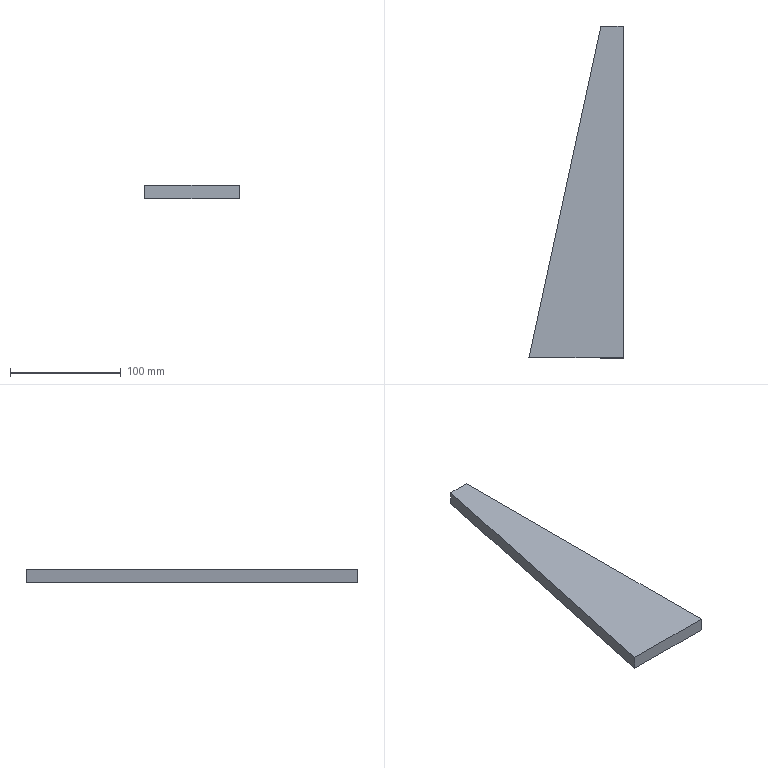Part | SolidWorks | features Extrusion 1 | 1 solid | 6 faces | box 85 x 300 x 12 mm | volume 189000 mm3 | plane 6
STEP:
#1=CARTESIAN_POINT('',(-85.,0.,-6.));
#2=VERTEX_POINT('',#1);
#3=CARTESIAN_POINT('',(0.,0.,-6.));
#4=VERTEX_POINT('',#3);
#5=CARTESIAN_POINT('',(0.,0.,-6.));
#6=DIRECTION('',(1.,0.,0.));
#7=VECTOR('',#6,1000.);
#8=LINE('',#5,#7);
#9=EDGE_CURVE('',#2,#4,#8,.T.);
#10=ORIENTED_EDGE('',*,*,#9,.T.);
#11=CARTESIAN_POINT('',(0.,0.,6.));
#12=VERTEX_POINT('',#11);
#13=CARTESIAN_POINT('',(0.,0.,6.));
#14=DIRECTION('',(0.,0.,-1.));
#15=VECTOR('',#14,1000.);
#16=LINE('',#13,#15);
#17=EDGE_CURVE('',#12,#4,#16,.T.);
#18=ORIENTED_EDGE('',*,*,#17,.F.);
#19=CARTESIAN_POINT('',(-85.,0.,6.));
#20=VERTEX_POINT('',#19);
#21=CARTESIAN_POINT('',(0.,0.,6.));
#22=DIRECTION('',(1.,0.,0.));
#23=VECTOR('',#22,1000.);
#24=LINE('',#21,#23);
#25=EDGE_CURVE('',#20,#12,#24,.T.);
#26=ORIENTED_EDGE('',*,*,#25,.F.);
#27=CARTESIAN_POINT('',(-85.,0.,6.));
#28=DIRECTION('',(0.,0.,-1.));
#29=VECTOR('',#28,1000.);
#30=LINE('',#27,#29);
#31=EDGE_CURVE('',#20,#2,#30,.T.);
#32=ORIENTED_EDGE('',*,*,#31,.T.);
#33=EDGE_LOOP('',(#10,#18,#26,#32));
#34=FACE_OUTER_BOUND('',#33,.T.);
#35=CARTESIAN_POINT('',(0.,0.,6.));
#36=DIRECTION('',(0.,1.,0.));
#37=DIRECTION('',(-1.,0.,0.));
#38=AXIS2_PLACEMENT_3D('',#35,#36,#37);
#39=PLANE('',#38);
#40=ADVANCED_FACE('',(#34),#39,.F.);
#41=CARTESIAN_POINT('',(0.,300.,-6.));
#42=VERTEX_POINT('',#41);
#43=CARTESIAN_POINT('',(0.,0.,-6.));
#44=DIRECTION('',(0.,1.,0.));
#45=VECTOR('',#44,1000.);
#46=LINE('',#43,#45);
#47=EDGE_CURVE('',#4,#42,#46,.T.);
#48=ORIENTED_EDGE('',*,*,#47,.T.);
#49=CARTESIAN_POINT('',(0.,300.,6.));
#50=VERTEX_POINT('',#49);
#51=CARTESIAN_POINT('',(0.,300.,6.));
#52=DIRECTION('',(0.,0.,-1.));
#53=VECTOR('',#52,1000.);
#54=LINE('',#51,#53);
#55=EDGE_CURVE('',#50,#42,#54,.T.);
#56=ORIENTED_EDGE('',*,*,#55,.F.);
#57=CARTESIAN_POINT('',(0.,0.,6.));
#58=DIRECTION('',(0.,1.,0.));
#59=VECTOR('',#58,1000.);
#60=LINE('',#57,#59);
#61=EDGE_CURVE('',#12,#50,#60,.T.);
#62=ORIENTED_EDGE('',*,*,#61,.F.);
#63=ORIENTED_EDGE('',*,*,#17,.T.);
#64=EDGE_LOOP('',(#48,#56,#62,#63));
#65=FACE_OUTER_BOUND('',#64,.T.);
#66=CARTESIAN_POINT('',(0.,0.,6.));
#67=DIRECTION('',(-1.,0.,0.));
#68=DIRECTION('',(0.,0.,1.));
#69=AXIS2_PLACEMENT_3D('',#66,#67,#68);
#70=PLANE('',#69);
#71=ADVANCED_FACE('',(#65),#70,.F.);
#72=CARTESIAN_POINT('',(-20.,300.,-6.));
#73=VERTEX_POINT('',#72);
#74=CARTESIAN_POINT('',(0.,300.,-6.));
#75=DIRECTION('',(-1.,0.,0.));
#76=VECTOR('',#75,1000.);
#77=LINE('',#74,#76);
#78=EDGE_CURVE('',#42,#73,#77,.T.);
#79=ORIENTED_EDGE('',*,*,#78,.T.);
#80=CARTESIAN_POINT('',(-20.,300.,6.));
#81=VERTEX_POINT('',#80);
#82=CARTESIAN_POINT('',(-20.,300.,6.));
#83=DIRECTION('',(0.,0.,-1.));
#84=VECTOR('',#83,1000.);
#85=LINE('',#82,#84);
#86=EDGE_CURVE('',#81,#73,#85,.T.);
#87=ORIENTED_EDGE('',*,*,#86,.F.);
#88=CARTESIAN_POINT('',(0.,300.,6.));
#89=DIRECTION('',(-1.,0.,0.));
#90=VECTOR('',#89,1000.);
#91=LINE('',#88,#90);
#92=EDGE_CURVE('',#50,#81,#91,.T.);
#93=ORIENTED_EDGE('',*,*,#92,.F.);
#94=ORIENTED_EDGE('',*,*,#55,.T.);
#95=EDGE_LOOP('',(#79,#87,#93,#94));
#96=FACE_OUTER_BOUND('',#95,.T.);
#97=CARTESIAN_POINT('',(0.,300.,6.));
#98=DIRECTION('',(0.,-1.,0.));
#99=DIRECTION('',(0.,0.,-1.));
#100=AXIS2_PLACEMENT_3D('',#97,#98,#99);
#101=PLANE('',#100);
#102=ADVANCED_FACE('',(#96),#101,.F.);
#103=CARTESIAN_POINT('',(-20.,300.,-6.));
#104=DIRECTION('',(-0.2118,-0.9773,0.));
#105=VECTOR('',#104,1000.);
#106=LINE('',#103,#105);
#107=EDGE_CURVE('',#73,#2,#106,.T.);
#108=ORIENTED_EDGE('',*,*,#107,.T.);
#109=ORIENTED_EDGE('',*,*,#31,.F.);
#110=CARTESIAN_POINT('',(-20.,300.,6.));
#111=DIRECTION('',(-0.2118,-0.9773,0.));
#112=VECTOR('',#111,1000.);
#113=LINE('',#110,#112);
#114=EDGE_CURVE('',#81,#20,#113,.T.);
#115=ORIENTED_EDGE('',*,*,#114,.F.);
#116=ORIENTED_EDGE('',*,*,#86,.T.);
#117=EDGE_LOOP('',(#108,#109,#115,#116));
#118=FACE_OUTER_BOUND('',#117,.T.);
#119=CARTESIAN_POINT('',(-20.,300.,6.));
#120=DIRECTION('',(0.9773,-0.2118,0.));
#121=DIRECTION('',(0.2118,0.9773,0.));
#122=AXIS2_PLACEMENT_3D('',#119,#120,#121);
#123=PLANE('',#122);
#124=ADVANCED_FACE('',(#118),#123,.F.);
#125=ORIENTED_EDGE('',*,*,#25,.T.);
#126=ORIENTED_EDGE('',*,*,#61,.T.);
#127=ORIENTED_EDGE('',*,*,#92,.T.);
#128=ORIENTED_EDGE('',*,*,#114,.T.);
#129=EDGE_LOOP('',(#125,#126,#127,#128));
#130=FACE_OUTER_BOUND('',#129,.T.);
#131=CARTESIAN_POINT('',(0.,0.,6.));
#132=DIRECTION('',(0.,0.,-1.));
#133=DIRECTION('',(-1.,0.,0.));
#134=AXIS2_PLACEMENT_3D('',#131,#132,#133);
#135=PLANE('',#134);
#136=ADVANCED_FACE('',(#130),#135,.F.);
#137=ORIENTED_EDGE('',*,*,#9,.F.);
#138=ORIENTED_EDGE('',*,*,#107,.F.);
#139=ORIENTED_EDGE('',*,*,#78,.F.);
#140=ORIENTED_EDGE('',*,*,#47,.F.);
#141=EDGE_LOOP('',(#137,#138,#139,#140));
#142=FACE_OUTER_BOUND('',#141,.T.);
#143=CARTESIAN_POINT('',(0.,0.,-6.));
#144=DIRECTION('',(0.,0.,-1.));
#145=DIRECTION('',(-1.,0.,0.));
#146=AXIS2_PLACEMENT_3D('',#143,#144,#145);
#147=PLANE('',#146);
#148=ADVANCED_FACE('',(#142),#147,.T.);
#149=CLOSED_SHELL('',(#40,#71,#102,#124,#136,#148));
#150=MANIFOLD_SOLID_BREP('',#149);
#151=CARTESIAN_POINT('',(0.,0.,0.));
#152=DIRECTION('',(0.,0.,1.));
#153=DIRECTION('',(1.,0.,0.));
#154=AXIS2_PLACEMENT_3D('',#151,#152,#153);
#155=(LENGTH_UNIT()NAMED_UNIT(*)SI_UNIT(.MILLI.,.METRE.));
#156=UNCERTAINTY_MEASURE_WITH_UNIT(LENGTH_MEASURE(0.00001),#155,'','');
#157=(NAMED_UNIT(*)PLANE_ANGLE_UNIT()SI_UNIT($,.RADIAN.));
#158=(NAMED_UNIT(*)SI_UNIT($,.STERADIAN.)SOLID_ANGLE_UNIT());
#159=(GEOMETRIC_REPRESENTATION_CONTEXT(3)GLOBAL_UNCERTAINTY_ASSIGNED_CONTEXT((#156))GLOBAL_UNIT_ASSIGNED_CONTEXT((#155,#157,#158))REPRESENTATION_CONTEXT('',''));
#160=ADVANCED_BREP_SHAPE_REPRESENTATION('',(#150,#154),#159);